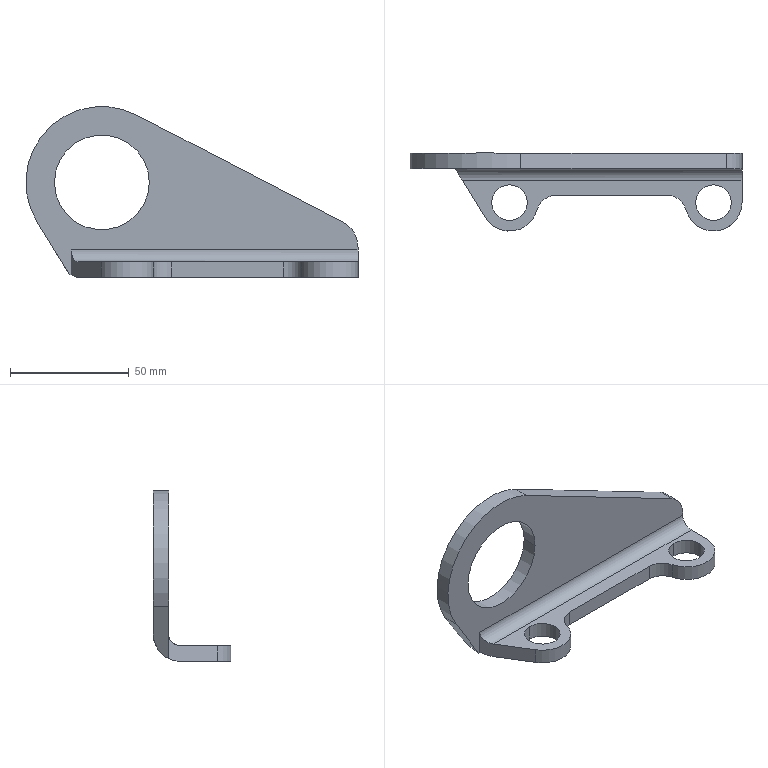Part | SolidWorks | features BaseBody 1 | 1 solid | 23 faces | box 140 x 32.8 x 72 mm | volume 44533 mm3 | cylinder 14 | plane 9 | commonest cylinder face diameters 15 x4 24 x3 16 x2 40 x2 10 x1 23 x1
STEP:
#1=CARTESIAN_POINT('',(-33.,576.8,478.15));
#2=VERTEX_POINT('',#1);
#3=CARTESIAN_POINT('',(-73.,576.8,478.15));
#4=VERTEX_POINT('',#3);
#5=CARTESIAN_POINT('',(-53.,576.8,478.15));
#6=DIRECTION('',(0.,1.,0.));
#7=DIRECTION('',(-1.,0.,0.));
#8=AXIS2_PLACEMENT_3D('',#5,#6,#7);
#9=CIRCLE('',#8,20.);
#10=EDGE_CURVE('',#2,#4,#9,.T.);
#11=ORIENTED_EDGE('',*,*,#10,.T.);
#12=CARTESIAN_POINT('',(-73.,570.3,478.15));
#13=VERTEX_POINT('',#12);
#14=CARTESIAN_POINT('',(-73.,576.8,478.15));
#15=DIRECTION('',(0.,-1.,0.));
#16=VECTOR('',#15,1000.);
#17=LINE('',#14,#16);
#18=EDGE_CURVE('',#4,#13,#17,.T.);
#19=ORIENTED_EDGE('',*,*,#18,.T.);
#20=CARTESIAN_POINT('',(-33.,570.3,478.15));
#21=VERTEX_POINT('',#20);
#22=CARTESIAN_POINT('',(-53.,570.3,478.15));
#23=DIRECTION('',(0.,1.,0.));
#24=DIRECTION('',(-1.,0.,0.));
#25=AXIS2_PLACEMENT_3D('',#22,#23,#24);
#26=CIRCLE('',#25,20.);
#27=EDGE_CURVE('',#21,#13,#26,.T.);
#28=ORIENTED_EDGE('',*,*,#27,.F.);
#29=CARTESIAN_POINT('',(-33.,576.8,478.15));
#30=DIRECTION('',(0.,-1.,0.));
#31=VECTOR('',#30,1000.);
#32=LINE('',#29,#31);
#33=EDGE_CURVE('',#2,#21,#32,.T.);
#34=ORIENTED_EDGE('',*,*,#33,.F.);
#35=EDGE_LOOP('',(#11,#19,#28,#34));
#36=FACE_OUTER_BOUND('',#35,.T.);
#37=CARTESIAN_POINT('',(-53.,576.8,478.15));
#38=DIRECTION('',(0.,-1.,0.));
#39=DIRECTION('',(1.,0.,0.));
#40=AXIS2_PLACEMENT_3D('',#37,#38,#39);
#41=CYLINDRICAL_SURFACE('',#40,20.);
#42=ADVANCED_FACE('',(#36),#41,.F.);
#43=CARTESIAN_POINT('',(43.,563.5,438.15));
#44=VERTEX_POINT('',#43);
#45=CARTESIAN_POINT('',(43.,548.5,438.15));
#46=VERTEX_POINT('',#45);
#47=CARTESIAN_POINT('',(43.,556.,438.15));
#48=DIRECTION('',(0.,0.,-1.));
#49=DIRECTION('',(-1.,0.,0.));
#50=AXIS2_PLACEMENT_3D('',#47,#48,#49);
#51=CIRCLE('',#50,7.5);
#52=EDGE_CURVE('',#44,#46,#51,.T.);
#53=ORIENTED_EDGE('',*,*,#52,.T.);
#54=CARTESIAN_POINT('',(43.,548.5,444.65));
#55=VERTEX_POINT('',#54);
#56=CARTESIAN_POINT('',(43.,548.5,438.15));
#57=DIRECTION('',(0.,0.,1.));
#58=VECTOR('',#57,1000.);
#59=LINE('',#56,#58);
#60=EDGE_CURVE('',#46,#55,#59,.T.);
#61=ORIENTED_EDGE('',*,*,#60,.T.);
#62=CARTESIAN_POINT('',(43.,563.5,444.65));
#63=VERTEX_POINT('',#62);
#64=CARTESIAN_POINT('',(43.,556.,444.65));
#65=DIRECTION('',(0.,0.,-1.));
#66=DIRECTION('',(-1.,0.,0.));
#67=AXIS2_PLACEMENT_3D('',#64,#65,#66);
#68=CIRCLE('',#67,7.5);
#69=EDGE_CURVE('',#63,#55,#68,.T.);
#70=ORIENTED_EDGE('',*,*,#69,.F.);
#71=CARTESIAN_POINT('',(43.,563.5,438.15));
#72=DIRECTION('',(0.,0.,1.));
#73=VECTOR('',#72,1000.);
#74=LINE('',#71,#73);
#75=EDGE_CURVE('',#44,#63,#74,.T.);
#76=ORIENTED_EDGE('',*,*,#75,.F.);
#77=EDGE_LOOP('',(#53,#61,#70,#76));
#78=FACE_OUTER_BOUND('',#77,.T.);
#79=CARTESIAN_POINT('',(43.,556.,438.15));
#80=DIRECTION('',(0.,0.,1.));
#81=DIRECTION('',(0.,1.,0.));
#82=AXIS2_PLACEMENT_3D('',#79,#80,#81);
#83=CYLINDRICAL_SURFACE('',#82,7.5);
#84=ADVANCED_FACE('',(#78),#83,.F.);
#85=CARTESIAN_POINT('',(-43.,563.5,438.15));
#86=VERTEX_POINT('',#85);
#87=CARTESIAN_POINT('',(-43.,548.5,438.15));
#88=VERTEX_POINT('',#87);
#89=CARTESIAN_POINT('',(-43.,556.,438.15));
#90=DIRECTION('',(0.,0.,-1.));
#91=DIRECTION('',(-1.,0.,0.));
#92=AXIS2_PLACEMENT_3D('',#89,#90,#91);
#93=CIRCLE('',#92,7.5);
#94=EDGE_CURVE('',#86,#88,#93,.T.);
#95=ORIENTED_EDGE('',*,*,#94,.T.);
#96=CARTESIAN_POINT('',(-43.,548.5,444.65));
#97=VERTEX_POINT('',#96);
#98=CARTESIAN_POINT('',(-43.,548.5,438.15));
#99=DIRECTION('',(0.,0.,1.));
#100=VECTOR('',#99,1000.);
#101=LINE('',#98,#100);
#102=EDGE_CURVE('',#88,#97,#101,.T.);
#103=ORIENTED_EDGE('',*,*,#102,.T.);
#104=CARTESIAN_POINT('',(-43.,563.5,444.65));
#105=VERTEX_POINT('',#104);
#106=CARTESIAN_POINT('',(-43.,556.,444.65));
#107=DIRECTION('',(0.,0.,-1.));
#108=DIRECTION('',(-1.,0.,0.));
#109=AXIS2_PLACEMENT_3D('',#106,#107,#108);
#110=CIRCLE('',#109,7.5);
#111=EDGE_CURVE('',#105,#97,#110,.T.);
#112=ORIENTED_EDGE('',*,*,#111,.F.);
#113=CARTESIAN_POINT('',(-43.,563.5,438.15));
#114=DIRECTION('',(0.,0.,1.));
#115=VECTOR('',#114,1000.);
#116=LINE('',#113,#115);
#117=EDGE_CURVE('',#86,#105,#116,.T.);
#118=ORIENTED_EDGE('',*,*,#117,.F.);
#119=EDGE_LOOP('',(#95,#103,#112,#118));
#120=FACE_OUTER_BOUND('',#119,.T.);
#121=CARTESIAN_POINT('',(-43.,556.,438.15));
#122=DIRECTION('',(0.,0.,1.));
#123=DIRECTION('',(0.,1.,0.));
#124=AXIS2_PLACEMENT_3D('',#121,#122,#123);
#125=CYLINDRICAL_SURFACE('',#124,7.5);
#126=ADVANCED_FACE('',(#120),#125,.F.);
#127=CARTESIAN_POINT('',(55.,565.3,438.15));
#128=VERTEX_POINT('',#127);
#129=CARTESIAN_POINT('',(55.,576.8,449.65));
#130=VERTEX_POINT('',#129);
#131=CARTESIAN_POINT('',(55.,565.3,449.65));
#132=DIRECTION('',(1.,0.,0.));
#133=DIRECTION('',(0.,1.,0.));
#134=AXIS2_PLACEMENT_3D('',#131,#132,#133);
#135=CIRCLE('',#134,11.5);
#136=EDGE_CURVE('',#128,#130,#135,.T.);
#137=ORIENTED_EDGE('',*,*,#136,.F.);
#138=CARTESIAN_POINT('',(-62.838,565.3,438.15));
#139=VERTEX_POINT('',#138);
#140=CARTESIAN_POINT('',(55.,565.3,438.15));
#141=DIRECTION('',(1.,0.,0.));
#142=VECTOR('',#141,1000.);
#143=LINE('',#140,#142);
#144=EDGE_CURVE('',#139,#128,#143,.T.);
#145=ORIENTED_EDGE('',*,*,#144,.F.);
#146=CARTESIAN_POINT('',(-65.922,570.3,439.294));
#147=VERTEX_POINT('',#146);
#148=CARTESIAN_POINT('',(-65.922,570.3,439.294));
#149=CARTESIAN_POINT('',(-64.956,568.734,438.538));
#150=CARTESIAN_POINT('',(-63.91,567.039,438.15));
#151=CARTESIAN_POINT('',(-62.838,565.3,438.15));
#152=(BOUNDED_CURVE()B_SPLINE_CURVE(3,(#148,#149,#150,#151),.UNSPECIFIED.,.F.,.F.)B_SPLINE_CURVE_WITH_KNOTS((4,4),(4.263,4.712),.UNSPECIFIED.)CURVE()GEOMETRIC_REPRESENTATION_ITEM()RATIONAL_B_SPLINE_CURVE((1.,0.9832,0.9832,1.))REPRESENTATION_ITEM(''));
#153=EDGE_CURVE('',#147,#139,#152,.T.);
#154=ORIENTED_EDGE('',*,*,#153,.F.);
#155=CARTESIAN_POINT('',(-66.628,570.3,439.294));
#156=VERTEX_POINT('',#155);
#157=CARTESIAN_POINT('',(-66.628,570.3,439.294));
#158=DIRECTION('',(1.,0.,0.));
#159=VECTOR('',#158,1000.);
#160=LINE('',#157,#159);
#161=EDGE_CURVE('',#156,#147,#160,.T.);
#162=ORIENTED_EDGE('',*,*,#161,.F.);
#163=CARTESIAN_POINT('',(-73.017,576.8,449.65));
#164=VERTEX_POINT('',#163);
#165=CARTESIAN_POINT('',(-73.017,576.8,449.65));
#166=CARTESIAN_POINT('',(-70.217,576.8,445.111));
#167=CARTESIAN_POINT('',(-67.845,574.387,441.267));
#168=CARTESIAN_POINT('',(-66.628,570.3,439.294));
#169=(BOUNDED_CURVE()B_SPLINE_CURVE(3,(#165,#166,#167,#168),.UNSPECIFIED.,.F.,.F.)B_SPLINE_CURVE_WITH_KNOTS((4,4),(4.712,5.833),.UNSPECIFIED.)CURVE()GEOMETRIC_REPRESENTATION_ITEM()RATIONAL_B_SPLINE_CURVE((1.,0.898,0.898,1.))REPRESENTATION_ITEM(''));
#170=EDGE_CURVE('',#164,#156,#169,.T.);
#171=ORIENTED_EDGE('',*,*,#170,.F.);
#172=CARTESIAN_POINT('',(-65.922,576.8,449.65));
#173=DIRECTION('',(-1.,0.,0.));
#174=VECTOR('',#173,1000.);
#175=LINE('',#172,#174);
#176=EDGE_CURVE('',#130,#164,#175,.T.);
#177=ORIENTED_EDGE('',*,*,#176,.F.);
#178=EDGE_LOOP('',(#137,#145,#154,#162,#171,#177));
#179=FACE_OUTER_BOUND('',#178,.T.);
#180=CARTESIAN_POINT('',(-53.,565.3,449.65));
#181=DIRECTION('',(1.,0.,0.));
#182=DIRECTION('',(0.,0.,-1.));
#183=AXIS2_PLACEMENT_3D('',#180,#181,#182);
#184=CYLINDRICAL_SURFACE('',#183,11.5);
#185=ADVANCED_FACE('',(#179),#184,.T.);
#186=CARTESIAN_POINT('',(55.,570.3,449.65));
#187=VERTEX_POINT('',#186);
#188=CARTESIAN_POINT('',(55.,565.3,444.65));
#189=VERTEX_POINT('',#188);
#190=CARTESIAN_POINT('',(55.,565.3,449.65));
#191=DIRECTION('',(-1.,0.,0.));
#192=DIRECTION('',(0.,1.,0.));
#193=AXIS2_PLACEMENT_3D('',#190,#191,#192);
#194=CIRCLE('',#193,5.);
#195=EDGE_CURVE('',#187,#189,#194,.T.);
#196=ORIENTED_EDGE('',*,*,#195,.F.);
#197=CARTESIAN_POINT('',(-65.922,570.3,449.65));
#198=VERTEX_POINT('',#197);
#199=CARTESIAN_POINT('',(55.,570.3,449.65));
#200=DIRECTION('',(1.,0.,0.));
#201=VECTOR('',#200,1000.);
#202=LINE('',#199,#201);
#203=EDGE_CURVE('',#198,#187,#202,.T.);
#204=ORIENTED_EDGE('',*,*,#203,.F.);
#205=CARTESIAN_POINT('',(-62.838,565.3,444.65));
#206=VERTEX_POINT('',#205);
#207=CARTESIAN_POINT('',(-62.838,565.3,444.65));
#208=CARTESIAN_POINT('',(-64.644,568.229,444.65));
#209=CARTESIAN_POINT('',(-65.922,570.3,446.721));
#210=CARTESIAN_POINT('',(-65.922,570.3,449.65));
#211=(BOUNDED_CURVE()B_SPLINE_CURVE(3,(#207,#208,#209,#210),.UNSPECIFIED.,.F.,.F.)B_SPLINE_CURVE_WITH_KNOTS((4,4),(1.571,3.142),.UNSPECIFIED.)CURVE()GEOMETRIC_REPRESENTATION_ITEM()RATIONAL_B_SPLINE_CURVE((1.,0.8047,0.8047,1.))REPRESENTATION_ITEM(''));
#212=EDGE_CURVE('',#206,#198,#211,.T.);
#213=ORIENTED_EDGE('',*,*,#212,.F.);
#214=CARTESIAN_POINT('',(-65.922,565.3,444.65));
#215=DIRECTION('',(-1.,0.,0.));
#216=VECTOR('',#215,1000.);
#217=LINE('',#214,#216);
#218=EDGE_CURVE('',#189,#206,#217,.T.);
#219=ORIENTED_EDGE('',*,*,#218,.F.);
#220=EDGE_LOOP('',(#196,#204,#213,#219));
#221=FACE_OUTER_BOUND('',#220,.T.);
#222=CARTESIAN_POINT('',(43.,565.3,449.65));
#223=DIRECTION('',(1.,0.,0.));
#224=DIRECTION('',(0.,1.,0.));
#225=AXIS2_PLACEMENT_3D('',#222,#223,#224);
#226=CYLINDRICAL_SURFACE('',#225,5.);
#227=ADVANCED_FACE('',(#221),#226,.F.);
#228=ORIENTED_EDGE('',*,*,#102,.F.);
#229=CARTESIAN_POINT('',(-43.,556.,438.15));
#230=DIRECTION('',(0.,0.,-1.));
#231=DIRECTION('',(-1.,0.,0.));
#232=AXIS2_PLACEMENT_3D('',#229,#230,#231);
#233=CIRCLE('',#232,7.5);
#234=EDGE_CURVE('',#88,#86,#233,.T.);
#235=ORIENTED_EDGE('',*,*,#234,.T.);
#236=ORIENTED_EDGE('',*,*,#117,.T.);
#237=CARTESIAN_POINT('',(-43.,556.,444.65));
#238=DIRECTION('',(0.,0.,-1.));
#239=DIRECTION('',(-1.,0.,0.));
#240=AXIS2_PLACEMENT_3D('',#237,#238,#239);
#241=CIRCLE('',#240,7.5);
#242=EDGE_CURVE('',#97,#105,#241,.T.);
#243=ORIENTED_EDGE('',*,*,#242,.F.);
#244=EDGE_LOOP('',(#228,#235,#236,#243));
#245=FACE_OUTER_BOUND('',#244,.T.);
#246=CARTESIAN_POINT('',(-43.,556.,438.15));
#247=DIRECTION('',(0.,0.,1.));
#248=DIRECTION('',(0.,1.,0.));
#249=AXIS2_PLACEMENT_3D('',#246,#247,#248);
#250=CYLINDRICAL_SURFACE('',#249,7.5);
#251=ADVANCED_FACE('',(#245),#250,.F.);
#252=ORIENTED_EDGE('',*,*,#60,.F.);
#253=CARTESIAN_POINT('',(43.,556.,438.15));
#254=DIRECTION('',(0.,0.,-1.));
#255=DIRECTION('',(-1.,0.,0.));
#256=AXIS2_PLACEMENT_3D('',#253,#254,#255);
#257=CIRCLE('',#256,7.5);
#258=EDGE_CURVE('',#46,#44,#257,.T.);
#259=ORIENTED_EDGE('',*,*,#258,.T.);
#260=ORIENTED_EDGE('',*,*,#75,.T.);
#261=CARTESIAN_POINT('',(43.,556.,444.65));
#262=DIRECTION('',(0.,0.,-1.));
#263=DIRECTION('',(-1.,0.,0.));
#264=AXIS2_PLACEMENT_3D('',#261,#262,#263);
#265=CIRCLE('',#264,7.5);
#266=EDGE_CURVE('',#55,#63,#265,.T.);
#267=ORIENTED_EDGE('',*,*,#266,.F.);
#268=EDGE_LOOP('',(#252,#259,#260,#267));
#269=FACE_OUTER_BOUND('',#268,.T.);
#270=CARTESIAN_POINT('',(43.,556.,438.15));
#271=DIRECTION('',(0.,0.,1.));
#272=DIRECTION('',(0.,1.,0.));
#273=AXIS2_PLACEMENT_3D('',#270,#271,#272);
#274=CYLINDRICAL_SURFACE('',#273,7.5);
#275=ADVANCED_FACE('',(#269),#274,.F.);
#276=CARTESIAN_POINT('',(-65.922,570.3,438.15));
#277=DIRECTION('',(0.,0.,1.));
#278=VECTOR('',#277,1000.);
#279=LINE('',#276,#278);
#280=EDGE_CURVE('',#147,#198,#279,.T.);
#281=ORIENTED_EDGE('',*,*,#280,.F.);
#282=ORIENTED_EDGE('',*,*,#153,.T.);
#283=CARTESIAN_POINT('',(-53.213,549.699,438.15));
#284=VERTEX_POINT('',#283);
#285=CARTESIAN_POINT('',(-65.922,570.3,438.15));
#286=DIRECTION('',(0.5251,-0.8511,0.));
#287=VECTOR('',#286,1000.);
#288=LINE('',#285,#287);
#289=EDGE_CURVE('',#139,#284,#288,.T.);
#290=ORIENTED_EDGE('',*,*,#289,.T.);
#291=CARTESIAN_POINT('',(-53.213,549.699,444.65));
#292=VERTEX_POINT('',#291);
#293=CARTESIAN_POINT('',(-53.213,549.699,438.15));
#294=DIRECTION('',(0.,0.,1.));
#295=VECTOR('',#294,1000.);
#296=LINE('',#293,#295);
#297=EDGE_CURVE('',#284,#292,#296,.T.);
#298=ORIENTED_EDGE('',*,*,#297,.T.);
#299=CARTESIAN_POINT('',(-65.922,570.3,444.65));
#300=DIRECTION('',(0.5251,-0.8511,0.));
#301=VECTOR('',#300,1000.);
#302=LINE('',#299,#301);
#303=EDGE_CURVE('',#206,#292,#302,.T.);
#304=ORIENTED_EDGE('',*,*,#303,.F.);
#305=ORIENTED_EDGE('',*,*,#212,.T.);
#306=EDGE_LOOP('',(#281,#282,#290,#298,#304,#305));
#307=FACE_OUTER_BOUND('',#306,.T.);
#308=CARTESIAN_POINT('',(-65.922,570.3,438.15));
#309=DIRECTION('',(-0.8511,-0.5251,0.));
#310=DIRECTION('',(-0.5251,0.8511,0.));
#311=AXIS2_PLACEMENT_3D('',#308,#309,#310);
#312=PLANE('',#311);
#313=ADVANCED_FACE('',(#307),#312,.T.);
#314=CARTESIAN_POINT('',(-31.381,553.,444.65));
#315=VERTEX_POINT('',#314);
#316=CARTESIAN_POINT('',(-43.,556.,444.65));
#317=DIRECTION('',(0.,0.,-1.));
#318=DIRECTION('',(-1.,0.,0.));
#319=AXIS2_PLACEMENT_3D('',#316,#317,#318);
#320=CIRCLE('',#319,12.);
#321=EDGE_CURVE('',#315,#292,#320,.T.);
#322=ORIENTED_EDGE('',*,*,#321,.T.);
#323=ORIENTED_EDGE('',*,*,#297,.F.);
#324=CARTESIAN_POINT('',(-31.381,553.,438.15));
#325=VERTEX_POINT('',#324);
#326=CARTESIAN_POINT('',(-43.,556.,438.15));
#327=DIRECTION('',(0.,0.,-1.));
#328=DIRECTION('',(-1.,0.,0.));
#329=AXIS2_PLACEMENT_3D('',#326,#327,#328);
#330=CIRCLE('',#329,12.);
#331=EDGE_CURVE('',#325,#284,#330,.T.);
#332=ORIENTED_EDGE('',*,*,#331,.F.);
#333=CARTESIAN_POINT('',(-31.381,553.,438.15));
#334=DIRECTION('',(0.,0.,1.));
#335=VECTOR('',#334,1000.);
#336=LINE('',#333,#335);
#337=EDGE_CURVE('',#325,#315,#336,.T.);
#338=ORIENTED_EDGE('',*,*,#337,.T.);
#339=EDGE_LOOP('',(#322,#323,#332,#338));
#340=FACE_OUTER_BOUND('',#339,.T.);
#341=CARTESIAN_POINT('',(-43.,556.,438.15));
#342=DIRECTION('',(0.,0.,1.));
#343=DIRECTION('',(0.,1.,0.));
#344=AXIS2_PLACEMENT_3D('',#341,#342,#343);
#345=CYLINDRICAL_SURFACE('',#344,12.);
#346=ADVANCED_FACE('',(#340),#345,.T.);
#347=CARTESIAN_POINT('',(-23.635,559.,444.65));
#348=VERTEX_POINT('',#347);
#349=CARTESIAN_POINT('',(-23.635,551.,444.65));
#350=DIRECTION('',(0.,0.,-1.));
#351=DIRECTION('',(-1.,0.,0.));
#352=AXIS2_PLACEMENT_3D('',#349,#350,#351);
#353=CIRCLE('',#352,8.);
#354=EDGE_CURVE('',#315,#348,#353,.T.);
#355=ORIENTED_EDGE('',*,*,#354,.F.);
#356=ORIENTED_EDGE('',*,*,#337,.F.);
#357=CARTESIAN_POINT('',(-23.635,559.,438.15));
#358=VERTEX_POINT('',#357);
#359=CARTESIAN_POINT('',(-23.635,551.,438.15));
#360=DIRECTION('',(0.,0.,-1.));
#361=DIRECTION('',(-1.,0.,0.));
#362=AXIS2_PLACEMENT_3D('',#359,#360,#361);
#363=CIRCLE('',#362,8.);
#364=EDGE_CURVE('',#325,#358,#363,.T.);
#365=ORIENTED_EDGE('',*,*,#364,.T.);
#366=CARTESIAN_POINT('',(-23.635,559.,438.15));
#367=DIRECTION('',(0.,0.,1.));
#368=VECTOR('',#367,1000.);
#369=LINE('',#366,#368);
#370=EDGE_CURVE('',#358,#348,#369,.T.);
#371=ORIENTED_EDGE('',*,*,#370,.T.);
#372=EDGE_LOOP('',(#355,#356,#365,#371));
#373=FACE_OUTER_BOUND('',#372,.T.);
#374=CARTESIAN_POINT('',(-23.635,551.,438.15));
#375=DIRECTION('',(0.,0.,1.));
#376=DIRECTION('',(0.,1.,0.));
#377=AXIS2_PLACEMENT_3D('',#374,#375,#376);
#378=CYLINDRICAL_SURFACE('',#377,8.);
#379=ADVANCED_FACE('',(#373),#378,.F.);
#380=CARTESIAN_POINT('',(23.635,559.,444.65));
#381=VERTEX_POINT('',#380);
#382=CARTESIAN_POINT('',(23.635,559.,444.65));
#383=DIRECTION('',(-1.,0.,0.));
#384=VECTOR('',#383,1000.);
#385=LINE('',#382,#384);
#386=EDGE_CURVE('',#381,#348,#385,.T.);
#387=ORIENTED_EDGE('',*,*,#386,.T.);
#388=ORIENTED_EDGE('',*,*,#370,.F.);
#389=CARTESIAN_POINT('',(23.635,559.,438.15));
#390=VERTEX_POINT('',#389);
#391=CARTESIAN_POINT('',(23.635,559.,438.15));
#392=DIRECTION('',(-1.,0.,0.));
#393=VECTOR('',#392,1000.);
#394=LINE('',#391,#393);
#395=EDGE_CURVE('',#390,#358,#394,.T.);
#396=ORIENTED_EDGE('',*,*,#395,.F.);
#397=CARTESIAN_POINT('',(23.635,559.,438.15));
#398=DIRECTION('',(0.,0.,1.));
#399=VECTOR('',#398,1000.);
#400=LINE('',#397,#399);
#401=EDGE_CURVE('',#390,#381,#400,.T.);
#402=ORIENTED_EDGE('',*,*,#401,.T.);
#403=EDGE_LOOP('',(#387,#388,#396,#402));
#404=FACE_OUTER_BOUND('',#403,.T.);
#405=CARTESIAN_POINT('',(23.635,559.,438.15));
#406=DIRECTION('',(0.,1.,0.));
#407=DIRECTION('',(1.,0.,0.));
#408=AXIS2_PLACEMENT_3D('',#405,#406,#407);
#409=PLANE('',#408);
#410=ADVANCED_FACE('',(#404),#409,.F.);
#411=CARTESIAN_POINT('',(31.381,553.,444.65));
#412=VERTEX_POINT('',#411);
#413=CARTESIAN_POINT('',(23.635,551.,444.65));
#414=DIRECTION('',(0.,0.,-1.));
#415=DIRECTION('',(-1.,0.,0.));
#416=AXIS2_PLACEMENT_3D('',#413,#414,#415);
#417=CIRCLE('',#416,8.);
#418=EDGE_CURVE('',#381,#412,#417,.T.);
#419=ORIENTED_EDGE('',*,*,#418,.F.);
#420=ORIENTED_EDGE('',*,*,#401,.F.);
#421=CARTESIAN_POINT('',(31.381,553.,438.15));
#422=VERTEX_POINT('',#421);
#423=CARTESIAN_POINT('',(23.635,551.,438.15));
#424=DIRECTION('',(0.,0.,-1.));
#425=DIRECTION('',(-1.,0.,0.));
#426=AXIS2_PLACEMENT_3D('',#423,#424,#425);
#427=CIRCLE('',#426,8.);
#428=EDGE_CURVE('',#390,#422,#427,.T.);
#429=ORIENTED_EDGE('',*,*,#428,.T.);
#430=CARTESIAN_POINT('',(31.381,553.,438.15));
#431=DIRECTION('',(0.,0.,1.));
#432=VECTOR('',#431,1000.);
#433=LINE('',#430,#432);
#434=EDGE_CURVE('',#422,#412,#433,.T.);
#435=ORIENTED_EDGE('',*,*,#434,.T.);
#436=EDGE_LOOP('',(#419,#420,#429,#435));
#437=FACE_OUTER_BOUND('',#436,.T.);
#438=CARTESIAN_POINT('',(23.635,551.,438.15));
#439=DIRECTION('',(0.,0.,1.));
#440=DIRECTION('',(0.,1.,0.));
#441=AXIS2_PLACEMENT_3D('',#438,#439,#440);
#442=CYLINDRICAL_SURFACE('',#441,8.);
#443=ADVANCED_FACE('',(#437),#442,.F.);
#444=CARTESIAN_POINT('',(55.,556.,444.65));
#445=VERTEX_POINT('',#444);
#446=CARTESIAN_POINT('',(43.,556.,444.65));
#447=DIRECTION('',(0.,0.,-1.));
#448=DIRECTION('',(-1.,0.,0.));
#449=AXIS2_PLACEMENT_3D('',#446,#447,#448);
#450=CIRCLE('',#449,12.);
#451=EDGE_CURVE('',#445,#412,#450,.T.);
#452=ORIENTED_EDGE('',*,*,#451,.T.);
#453=ORIENTED_EDGE('',*,*,#434,.F.);
#454=CARTESIAN_POINT('',(55.,556.,438.15));
#455=VERTEX_POINT('',#454);
#456=CARTESIAN_POINT('',(43.,556.,438.15));
#457=DIRECTION('',(0.,0.,-1.));
#458=DIRECTION('',(-1.,0.,0.));
#459=AXIS2_PLACEMENT_3D('',#456,#457,#458);
#460=CIRCLE('',#459,12.);
#461=EDGE_CURVE('',#455,#422,#460,.T.);
#462=ORIENTED_EDGE('',*,*,#461,.F.);
#463=CARTESIAN_POINT('',(55.,556.,438.15));
#464=DIRECTION('',(0.,0.,1.));
#465=VECTOR('',#464,1000.);
#466=LINE('',#463,#465);
#467=EDGE_CURVE('',#455,#445,#466,.T.);
#468=ORIENTED_EDGE('',*,*,#467,.T.);
#469=EDGE_LOOP('',(#452,#453,#462,#468));
#470=FACE_OUTER_BOUND('',#469,.T.);
#471=CARTESIAN_POINT('',(43.,556.,438.15));
#472=DIRECTION('',(0.,0.,1.));
#473=DIRECTION('',(0.,1.,0.));
#474=AXIS2_PLACEMENT_3D('',#471,#472,#473);
#475=CYLINDRICAL_SURFACE('',#474,12.);
#476=ADVANCED_FACE('',(#470),#475,.T.);
#477=CARTESIAN_POINT('',(55.,556.,444.65));
#478=DIRECTION('',(0.,1.,0.));
#479=VECTOR('',#478,1000.);
#480=LINE('',#477,#479);
#481=EDGE_CURVE('',#445,#189,#480,.T.);
#482=ORIENTED_EDGE('',*,*,#481,.T.);
#483=ORIENTED_EDGE('',*,*,#218,.T.);
#484=ORIENTED_EDGE('',*,*,#303,.T.);
#485=ORIENTED_EDGE('',*,*,#321,.F.);
#486=ORIENTED_EDGE('',*,*,#354,.T.);
#487=ORIENTED_EDGE('',*,*,#386,.F.);
#488=ORIENTED_EDGE('',*,*,#418,.T.);
#489=ORIENTED_EDGE('',*,*,#451,.F.);
#490=EDGE_LOOP('',(#482,#483,#484,#485,#486,#487,#488,#489));
#491=FACE_OUTER_BOUND('',#490,.T.);
#492=ORIENTED_EDGE('',*,*,#111,.T.);
#493=ORIENTED_EDGE('',*,*,#242,.T.);
#494=EDGE_LOOP('',(#492,#493));
#495=FACE_BOUND('',#494,.T.);
#496=ORIENTED_EDGE('',*,*,#69,.T.);
#497=ORIENTED_EDGE('',*,*,#266,.T.);
#498=EDGE_LOOP('',(#496,#497));
#499=FACE_BOUND('',#498,.T.);
#500=CARTESIAN_POINT('',(43.,556.,444.65));
#501=DIRECTION('',(0.,0.,-1.));
#502=DIRECTION('',(0.,-1.,0.));
#503=AXIS2_PLACEMENT_3D('',#500,#501,#502);
#504=PLANE('',#503);
#505=ADVANCED_FACE('',(#491,#495,#499),#504,.F.);
#506=CARTESIAN_POINT('',(-80.234,570.3,461.348));
#507=VERTEX_POINT('',#506);
#508=CARTESIAN_POINT('',(-80.234,570.3,461.348));
#509=DIRECTION('',(0.5251,0.,-0.8511));
#510=VECTOR('',#509,1000.);
#511=LINE('',#508,#510);
#512=EDGE_CURVE('',#507,#156,#511,.T.);
#513=ORIENTED_EDGE('',*,*,#512,.T.);
#514=ORIENTED_EDGE('',*,*,#161,.T.);
#515=ORIENTED_EDGE('',*,*,#280,.T.);
#516=ORIENTED_EDGE('',*,*,#203,.T.);
#517=CARTESIAN_POINT('',(55.,570.3,450.858));
#518=VERTEX_POINT('',#517);
#519=CARTESIAN_POINT('',(55.,570.3,438.15));
#520=DIRECTION('',(0.,0.,1.));
#521=VECTOR('',#520,1000.);
#522=LINE('',#519,#521);
#523=EDGE_CURVE('',#187,#518,#522,.T.);
#524=ORIENTED_EDGE('',*,*,#523,.T.);
#525=CARTESIAN_POINT('',(48.528,570.3,461.509));
#526=VERTEX_POINT('',#525);
#527=CARTESIAN_POINT('',(43.,570.3,450.858));
#528=DIRECTION('',(0.,1.,0.));
#529=DIRECTION('',(-1.,0.,0.));
#530=AXIS2_PLACEMENT_3D('',#527,#528,#529);
#531=CIRCLE('',#530,12.);
#532=EDGE_CURVE('',#526,#518,#531,.T.);
#533=ORIENTED_EDGE('',*,*,#532,.F.);
#534=CARTESIAN_POINT('',(-38.259,570.3,506.552));
#535=VERTEX_POINT('',#534);
#536=CARTESIAN_POINT('',(48.528,570.3,461.509));
#537=DIRECTION('',(-0.8876,0.,0.4607));
#538=VECTOR('',#537,1000.);
#539=LINE('',#536,#538);
#540=EDGE_CURVE('',#526,#535,#539,.T.);
#541=ORIENTED_EDGE('',*,*,#540,.T.);
#542=CARTESIAN_POINT('',(-53.,570.3,478.15));
#543=DIRECTION('',(0.,1.,0.));
#544=DIRECTION('',(-1.,0.,0.));
#545=AXIS2_PLACEMENT_3D('',#542,#543,#544);
#546=CIRCLE('',#545,32.);
#547=EDGE_CURVE('',#507,#535,#546,.T.);
#548=ORIENTED_EDGE('',*,*,#547,.F.);
#549=EDGE_LOOP('',(#513,#514,#515,#516,#524,#533,#541,#548));
#550=FACE_OUTER_BOUND('',#549,.T.);
#551=ORIENTED_EDGE('',*,*,#27,.T.);
#552=CARTESIAN_POINT('',(-53.,570.3,478.15));
#553=DIRECTION('',(0.,1.,0.));
#554=DIRECTION('',(-1.,0.,0.));
#555=AXIS2_PLACEMENT_3D('',#552,#553,#554);
#556=CIRCLE('',#555,20.);
#557=EDGE_CURVE('',#13,#21,#556,.T.);
#558=ORIENTED_EDGE('',*,*,#557,.T.);
#559=EDGE_LOOP('',(#551,#558));
#560=FACE_BOUND('',#559,.T.);
#561=CARTESIAN_POINT('',(-53.,570.3,478.15));
#562=DIRECTION('',(0.,1.,0.));
#563=DIRECTION('',(1.,0.,0.));
#564=AXIS2_PLACEMENT_3D('',#561,#562,#563);
#565=PLANE('',#564);
#566=ADVANCED_FACE('',(#550,#560),#565,.F.);
#567=ORIENTED_EDGE('',*,*,#10,.F.);
#568=CARTESIAN_POINT('',(-53.,576.8,478.15));
#569=DIRECTION('',(0.,1.,0.));
#570=DIRECTION('',(-1.,0.,0.));
#571=AXIS2_PLACEMENT_3D('',#568,#569,#570);
#572=CIRCLE('',#571,20.);
#573=EDGE_CURVE('',#4,#2,#572,.T.);
#574=ORIENTED_EDGE('',*,*,#573,.F.);
#575=EDGE_LOOP('',(#567,#574));
#576=FACE_BOUND('',#575,.T.);
#577=CARTESIAN_POINT('',(55.,576.8,450.858));
#578=VERTEX_POINT('',#577);
#579=CARTESIAN_POINT('',(55.,576.8,438.15));
#580=DIRECTION('',(0.,0.,1.));
#581=VECTOR('',#580,1000.);
#582=LINE('',#579,#581);
#583=EDGE_CURVE('',#130,#578,#582,.T.);
#584=ORIENTED_EDGE('',*,*,#583,.F.);
#585=ORIENTED_EDGE('',*,*,#176,.T.);
#586=CARTESIAN_POINT('',(-80.234,576.8,461.348));
#587=VERTEX_POINT('',#586);
#588=CARTESIAN_POINT('',(-80.234,576.8,461.348));
#589=DIRECTION('',(0.5251,0.,-0.8511));
#590=VECTOR('',#589,1000.);
#591=LINE('',#588,#590);
#592=EDGE_CURVE('',#587,#164,#591,.T.);
#593=ORIENTED_EDGE('',*,*,#592,.F.);
#594=CARTESIAN_POINT('',(-38.259,576.8,506.552));
#595=VERTEX_POINT('',#594);
#596=CARTESIAN_POINT('',(-53.,576.8,478.15));
#597=DIRECTION('',(0.,1.,0.));
#598=DIRECTION('',(-1.,0.,0.));
#599=AXIS2_PLACEMENT_3D('',#596,#597,#598);
#600=CIRCLE('',#599,32.);
#601=EDGE_CURVE('',#587,#595,#600,.T.);
#602=ORIENTED_EDGE('',*,*,#601,.T.);
#603=CARTESIAN_POINT('',(48.528,576.8,461.509));
#604=VERTEX_POINT('',#603);
#605=CARTESIAN_POINT('',(48.528,576.8,461.509));
#606=DIRECTION('',(-0.8876,0.,0.4607));
#607=VECTOR('',#606,1000.);
#608=LINE('',#605,#607);
#609=EDGE_CURVE('',#604,#595,#608,.T.);
#610=ORIENTED_EDGE('',*,*,#609,.F.);
#611=CARTESIAN_POINT('',(43.,576.8,450.858));
#612=DIRECTION('',(0.,1.,0.));
#613=DIRECTION('',(-1.,0.,0.));
#614=AXIS2_PLACEMENT_3D('',#611,#612,#613);
#615=CIRCLE('',#614,12.);
#616=EDGE_CURVE('',#604,#578,#615,.T.);
#617=ORIENTED_EDGE('',*,*,#616,.T.);
#618=EDGE_LOOP('',(#584,#585,#593,#602,#610,#617));
#619=FACE_OUTER_BOUND('',#618,.T.);
#620=CARTESIAN_POINT('',(-53.,576.8,478.15));
#621=DIRECTION('',(0.,1.,0.));
#622=DIRECTION('',(1.,0.,0.));
#623=AXIS2_PLACEMENT_3D('',#620,#621,#622);
#624=PLANE('',#623);
#625=ADVANCED_FACE('',(#576,#619),#624,.T.);
#626=ORIENTED_EDGE('',*,*,#592,.T.);
#627=ORIENTED_EDGE('',*,*,#170,.T.);
#628=ORIENTED_EDGE('',*,*,#512,.F.);
#629=CARTESIAN_POINT('',(-80.234,576.8,461.348));
#630=DIRECTION('',(0.,-1.,0.));
#631=VECTOR('',#630,1000.);
#632=LINE('',#629,#631);
#633=EDGE_CURVE('',#587,#507,#632,.T.);
#634=ORIENTED_EDGE('',*,*,#633,.F.);
#635=EDGE_LOOP('',(#626,#627,#628,#634));
#636=FACE_OUTER_BOUND('',#635,.T.);
#637=CARTESIAN_POINT('',(-80.234,576.8,461.348));
#638=DIRECTION('',(-0.8511,0.,-0.5251));
#639=DIRECTION('',(-0.5251,0.,0.8511));
#640=AXIS2_PLACEMENT_3D('',#637,#638,#639);
#641=PLANE('',#640);
#642=ADVANCED_FACE('',(#636),#641,.T.);
#643=ORIENTED_EDGE('',*,*,#18,.F.);
#644=ORIENTED_EDGE('',*,*,#573,.T.);
#645=ORIENTED_EDGE('',*,*,#33,.T.);
#646=ORIENTED_EDGE('',*,*,#557,.F.);
#647=EDGE_LOOP('',(#643,#644,#645,#646));
#648=FACE_OUTER_BOUND('',#647,.T.);
#649=CARTESIAN_POINT('',(-53.,576.8,478.15));
#650=DIRECTION('',(0.,-1.,0.));
#651=DIRECTION('',(1.,0.,0.));
#652=AXIS2_PLACEMENT_3D('',#649,#650,#651);
#653=CYLINDRICAL_SURFACE('',#652,20.);
#654=ADVANCED_FACE('',(#648),#653,.F.);
#655=ORIENTED_EDGE('',*,*,#94,.F.);
#656=ORIENTED_EDGE('',*,*,#234,.F.);
#657=EDGE_LOOP('',(#655,#656));
#658=FACE_BOUND('',#657,.T.);
#659=ORIENTED_EDGE('',*,*,#52,.F.);
#660=ORIENTED_EDGE('',*,*,#258,.F.);
#661=EDGE_LOOP('',(#659,#660));
#662=FACE_BOUND('',#661,.T.);
#663=ORIENTED_EDGE('',*,*,#289,.F.);
#664=ORIENTED_EDGE('',*,*,#144,.T.);
#665=CARTESIAN_POINT('',(55.,576.8,438.15));
#666=DIRECTION('',(0.,-1.,0.));
#667=VECTOR('',#666,1000.);
#668=LINE('',#665,#667);
#669=EDGE_CURVE('',#128,#455,#668,.T.);
#670=ORIENTED_EDGE('',*,*,#669,.T.);
#671=ORIENTED_EDGE('',*,*,#461,.T.);
#672=ORIENTED_EDGE('',*,*,#428,.F.);
#673=ORIENTED_EDGE('',*,*,#395,.T.);
#674=ORIENTED_EDGE('',*,*,#364,.F.);
#675=ORIENTED_EDGE('',*,*,#331,.T.);
#676=EDGE_LOOP('',(#663,#664,#670,#671,#672,#673,#674,#675));
#677=FACE_OUTER_BOUND('',#676,.T.);
#678=CARTESIAN_POINT('',(55.,576.8,438.15));
#679=DIRECTION('',(0.,0.,1.));
#680=DIRECTION('',(1.,0.,0.));
#681=AXIS2_PLACEMENT_3D('',#678,#679,#680);
#682=PLANE('',#681);
#683=ADVANCED_FACE('',(#658,#662,#677),#682,.F.);
#684=ORIENTED_EDGE('',*,*,#669,.F.);
#685=ORIENTED_EDGE('',*,*,#136,.T.);
#686=ORIENTED_EDGE('',*,*,#583,.T.);
#687=CARTESIAN_POINT('',(55.,576.8,450.858));
#688=DIRECTION('',(0.,-1.,0.));
#689=VECTOR('',#688,1000.);
#690=LINE('',#687,#689);
#691=EDGE_CURVE('',#578,#518,#690,.T.);
#692=ORIENTED_EDGE('',*,*,#691,.T.);
#693=ORIENTED_EDGE('',*,*,#523,.F.);
#694=ORIENTED_EDGE('',*,*,#195,.T.);
#695=ORIENTED_EDGE('',*,*,#481,.F.);
#696=ORIENTED_EDGE('',*,*,#467,.F.);
#697=EDGE_LOOP('',(#684,#685,#686,#692,#693,#694,#695,#696));
#698=FACE_OUTER_BOUND('',#697,.T.);
#699=CARTESIAN_POINT('',(55.,576.8,438.15));
#700=DIRECTION('',(1.,0.,0.));
#701=DIRECTION('',(0.,1.,0.));
#702=AXIS2_PLACEMENT_3D('',#699,#700,#701);
#703=PLANE('',#702);
#704=ADVANCED_FACE('',(#698),#703,.T.);
#705=ORIENTED_EDGE('',*,*,#532,.T.);
#706=ORIENTED_EDGE('',*,*,#691,.F.);
#707=ORIENTED_EDGE('',*,*,#616,.F.);
#708=CARTESIAN_POINT('',(48.528,576.8,461.509));
#709=DIRECTION('',(0.,-1.,0.));
#710=VECTOR('',#709,1000.);
#711=LINE('',#708,#710);
#712=EDGE_CURVE('',#604,#526,#711,.T.);
#713=ORIENTED_EDGE('',*,*,#712,.T.);
#714=EDGE_LOOP('',(#705,#706,#707,#713));
#715=FACE_OUTER_BOUND('',#714,.T.);
#716=CARTESIAN_POINT('',(43.,576.8,450.858));
#717=DIRECTION('',(0.,-1.,0.));
#718=DIRECTION('',(1.,0.,0.));
#719=AXIS2_PLACEMENT_3D('',#716,#717,#718);
#720=CYLINDRICAL_SURFACE('',#719,12.);
#721=ADVANCED_FACE('',(#715),#720,.T.);
#722=ORIENTED_EDGE('',*,*,#540,.F.);
#723=ORIENTED_EDGE('',*,*,#712,.F.);
#724=ORIENTED_EDGE('',*,*,#609,.T.);
#725=CARTESIAN_POINT('',(-38.259,576.8,506.552));
#726=DIRECTION('',(0.,-1.,0.));
#727=VECTOR('',#726,1000.);
#728=LINE('',#725,#727);
#729=EDGE_CURVE('',#595,#535,#728,.T.);
#730=ORIENTED_EDGE('',*,*,#729,.T.);
#731=EDGE_LOOP('',(#722,#723,#724,#730));
#732=FACE_OUTER_BOUND('',#731,.T.);
#733=CARTESIAN_POINT('',(48.528,576.8,461.509));
#734=DIRECTION('',(0.4607,0.,0.8876));
#735=DIRECTION('',(0.,-1.,0.));
#736=AXIS2_PLACEMENT_3D('',#733,#734,#735);
#737=PLANE('',#736);
#738=ADVANCED_FACE('',(#732),#737,.T.);
#739=ORIENTED_EDGE('',*,*,#547,.T.);
#740=ORIENTED_EDGE('',*,*,#729,.F.);
#741=ORIENTED_EDGE('',*,*,#601,.F.);
#742=ORIENTED_EDGE('',*,*,#633,.T.);
#743=EDGE_LOOP('',(#739,#740,#741,#742));
#744=FACE_OUTER_BOUND('',#743,.T.);
#745=CARTESIAN_POINT('',(-53.,576.8,478.15));
#746=DIRECTION('',(0.,-1.,0.));
#747=DIRECTION('',(1.,0.,0.));
#748=AXIS2_PLACEMENT_3D('',#745,#746,#747);
#749=CYLINDRICAL_SURFACE('',#748,32.);
#750=ADVANCED_FACE('',(#744),#749,.T.);
#751=CLOSED_SHELL('',(#42,#84,#126,#185,#227,#251,#275,#313,#346,#379,#410,#443,#476,#505,#566,#625,#642,#654,#683,#704,#721,#738,#750));
#752=MANIFOLD_SOLID_BREP('',#751);
#753=CARTESIAN_POINT('',(0.,0.,0.));
#754=DIRECTION('',(0.,0.,1.));
#755=DIRECTION('',(1.,0.,0.));
#756=AXIS2_PLACEMENT_3D('',#753,#754,#755);
#757=(LENGTH_UNIT()NAMED_UNIT(*)SI_UNIT(.MILLI.,.METRE.));
#758=UNCERTAINTY_MEASURE_WITH_UNIT(LENGTH_MEASURE(0.00001),#757,'','');
#759=(NAMED_UNIT(*)PLANE_ANGLE_UNIT()SI_UNIT($,.RADIAN.));
#760=(NAMED_UNIT(*)SI_UNIT($,.STERADIAN.)SOLID_ANGLE_UNIT());
#761=(GEOMETRIC_REPRESENTATION_CONTEXT(3)GLOBAL_UNCERTAINTY_ASSIGNED_CONTEXT((#758))GLOBAL_UNIT_ASSIGNED_CONTEXT((#757,#759,#760))REPRESENTATION_CONTEXT('',''));
#762=ADVANCED_BREP_SHAPE_REPRESENTATION('',(#752,#756),#761);